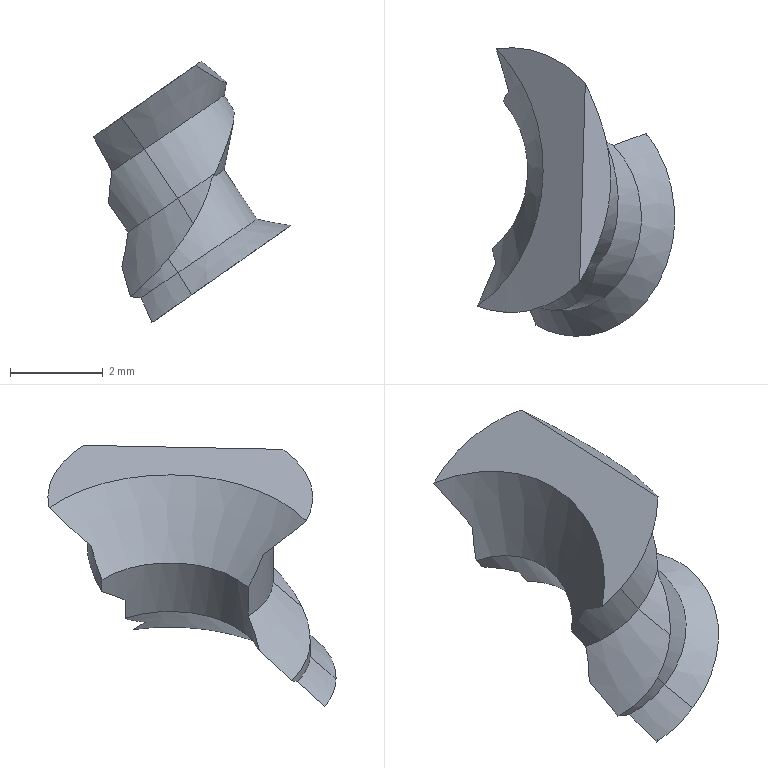Part | SolidWorks | features BaseBody 1 | 1 solid | 20 faces | box 4.246 x 6.208 x 5.627 mm | volume 24.691 mm3 | cone 11 | cylinder 6 | plane 3 | commonest cylinder face diameters 4 x6
STEP:
#1=CARTESIAN_POINT('',(-2079.786,537.162,-1636.577));
#2=VERTEX_POINT('',#1);
#3=CARTESIAN_POINT('',(-2078.265,541.527,-1635.512));
#4=VERTEX_POINT('',#3);
#5=CARTESIAN_POINT('',(-2079.786,537.162,-1636.577));
#6=CARTESIAN_POINT('',(-2079.49,537.155,-1636.37));
#7=CARTESIAN_POINT('',(-2079.24,537.225,-1636.195));
#8=CARTESIAN_POINT('',(-2078.948,537.352,-1635.991));
#9=CARTESIAN_POINT('',(-2078.864,537.398,-1635.931));
#10=CARTESIAN_POINT('',(-2078.755,537.466,-1635.855));
#11=CARTESIAN_POINT('',(-2078.722,537.489,-1635.832));
#12=CARTESIAN_POINT('',(-2078.677,537.521,-1635.8));
#13=CARTESIAN_POINT('',(-2078.655,537.537,-1635.785));
#14=CARTESIAN_POINT('',(-2078.631,537.555,-1635.768));
#15=CARTESIAN_POINT('',(-2078.62,537.564,-1635.76));
#16=CARTESIAN_POINT('',(-2078.615,537.568,-1635.757));
#17=CARTESIAN_POINT('',(-2078.612,537.57,-1635.755));
#18=CARTESIAN_POINT('',(-2078.612,537.57,-1635.755));
#19=CARTESIAN_POINT('',(-2078.419,537.723,-1635.62));
#20=CARTESIAN_POINT('',(-2078.258,537.904,-1635.507));
#21=CARTESIAN_POINT('',(-2078.061,538.198,-1635.369));
#22=CARTESIAN_POINT('',(-2078.003,538.299,-1635.328));
#23=CARTESIAN_POINT('',(-2077.926,538.455,-1635.275));
#24=CARTESIAN_POINT('',(-2077.903,538.507,-1635.258));
#25=CARTESIAN_POINT('',(-2077.87,538.586,-1635.235));
#26=CARTESIAN_POINT('',(-2077.854,538.626,-1635.224));
#27=CARTESIAN_POINT('',(-2077.839,538.665,-1635.214));
#28=CARTESIAN_POINT('',(-2077.829,538.692,-1635.207));
#29=CARTESIAN_POINT('',(-2077.825,538.704,-1635.204));
#30=CARTESIAN_POINT('',(-2077.738,538.953,-1635.143));
#31=CARTESIAN_POINT('',(-2077.686,539.201,-1635.106));
#32=CARTESIAN_POINT('',(-2077.653,539.579,-1635.084));
#33=CARTESIAN_POINT('',(-2077.65,539.706,-1635.082));
#34=CARTESIAN_POINT('',(-2077.657,539.895,-1635.086));
#35=CARTESIAN_POINT('',(-2077.663,539.989,-1635.091));
#36=CARTESIAN_POINT('',(-2077.676,540.098,-1635.099));
#37=CARTESIAN_POINT('',(-2077.682,540.145,-1635.104));
#38=CARTESIAN_POINT('',(-2077.686,540.176,-1635.107));
#39=CARTESIAN_POINT('',(-2077.689,540.193,-1635.109));
#40=CARTESIAN_POINT('',(-2077.727,540.434,-1635.135));
#41=CARTESIAN_POINT('',(-2077.79,540.666,-1635.18));
#42=CARTESIAN_POINT('',(-2077.98,541.116,-1635.313));
#43=CARTESIAN_POINT('',(-2078.106,541.333,-1635.401));
#44=CARTESIAN_POINT('',(-2078.265,541.527,-1635.512));
#45=B_SPLINE_CURVE_WITH_KNOTS('',3,(#5,#6,#7,#8,#9,#10,#11,#12,#13,#14,#15,#16,#17,#18,#19,#20,#21,#22,#23,#24,#25,#26,#27,#28,#29,#30,#31,#32,#33,#34,#35,#36,#37,#38,#39,#40,#41,#42,#43,#44),.UNSPECIFIED.,.F.,.F.,(4,2,2,2,1,1,1,2,2,2,2,2,1,2,2,2,2,1,1,2,2,2,4),(0.,0.125,0.1875,0.2188,0.2344,0.2422,0.2461,0.248,0.25,0.375,0.4375,0.4688,0.4844,0.4922,0.5,0.625,0.6875,0.7188,0.7344,0.7422,0.75,0.875,1.),.UNSPECIFIED.);
#46=EDGE_CURVE('',#2,#4,#45,.T.);
#47=ORIENTED_EDGE('',*,*,#46,.F.);
#48=CARTESIAN_POINT('',(-2080.638,537.403,-1637.174));
#49=VERTEX_POINT('',#48);
#50=CARTESIAN_POINT('',(-2080.638,537.403,-1637.174));
#51=CARTESIAN_POINT('',(-2080.371,537.25,-1636.987));
#52=CARTESIAN_POINT('',(-2080.079,537.168,-1636.782));
#53=CARTESIAN_POINT('',(-2079.786,537.162,-1636.577));
#54=B_SPLINE_CURVE_WITH_KNOTS('',3,(#50,#51,#52,#53),.UNSPECIFIED.,.F.,.F.,(4,4),(0.,1.),.UNSPECIFIED.);
#55=EDGE_CURVE('',#49,#2,#54,.T.);
#56=ORIENTED_EDGE('',*,*,#55,.F.);
#57=CARTESIAN_POINT('',(-2080.942,540.742,-1637.386));
#58=DIRECTION('',(0.5736,0.,-0.8192));
#59=DIRECTION('',(0.7965,0.2335,0.5577));
#60=AXIS2_PLACEMENT_3D('',#57,#58,#59);
#61=CIRCLE('',#60,3.36);
#62=EDGE_CURVE('',#4,#49,#61,.T.);
#63=ORIENTED_EDGE('',*,*,#62,.F.);
#64=EDGE_LOOP('',(#47,#56,#63));
#65=FACE_OUTER_BOUND('',#64,.T.);
#66=CARTESIAN_POINT('',(-2087.136,533.617,-1641.724));
#67=DIRECTION('',(0.5736,0.,-0.8192));
#68=DIRECTION('',(0.,-1.,0.));
#69=AXIS2_PLACEMENT_3D('',#66,#67,#68);
#70=PLANE('',#69);
#71=ADVANCED_FACE('',(#65),#70,.T.);
#72=CARTESIAN_POINT('',(-2078.976,541.269,-1635.356));
#73=VERTEX_POINT('',#72);
#74=CARTESIAN_POINT('',(-2080.286,541.707,-1635.267));
#75=VERTEX_POINT('',#74);
#76=CARTESIAN_POINT('',(-2078.976,541.269,-1635.356));
#77=CARTESIAN_POINT('',(-2079.333,541.497,-1635.327));
#78=CARTESIAN_POINT('',(-2079.782,541.661,-1635.306));
#79=CARTESIAN_POINT('',(-2080.286,541.707,-1635.267));
#80=B_SPLINE_CURVE_WITH_KNOTS('',3,(#76,#77,#78,#79),.UNSPECIFIED.,.F.,.F.,(4,4),(0.,1.),.UNSPECIFIED.);
#81=EDGE_CURVE('',#73,#75,#80,.T.);
#82=ORIENTED_EDGE('',*,*,#81,.F.);
#83=CARTESIAN_POINT('',(-2078.976,541.269,-1635.356));
#84=CARTESIAN_POINT('',(-2078.763,541.35,-1635.402));
#85=CARTESIAN_POINT('',(-2078.526,541.436,-1635.455));
#86=CARTESIAN_POINT('',(-2078.265,541.527,-1635.512));
#87=B_SPLINE_CURVE_WITH_KNOTS('',3,(#83,#84,#85,#86),.UNSPECIFIED.,.F.,.F.,(4,4),(0.,1.),.UNSPECIFIED.);
#88=EDGE_CURVE('',#73,#4,#87,.T.);
#89=ORIENTED_EDGE('',*,*,#88,.T.);
#90=ORIENTED_EDGE('',*,*,#62,.T.);
#91=CARTESIAN_POINT('',(-2080.873,538.001,-1636.635));
#92=VERTEX_POINT('',#91);
#93=CARTESIAN_POINT('',(-2080.873,538.001,-1636.635));
#94=CARTESIAN_POINT('',(-2080.806,537.825,-1636.792));
#95=CARTESIAN_POINT('',(-2080.728,537.626,-1636.971));
#96=CARTESIAN_POINT('',(-2080.638,537.403,-1637.174));
#97=B_SPLINE_CURVE_WITH_KNOTS('',3,(#93,#94,#95,#96),.UNSPECIFIED.,.F.,.F.,(4,4),(0.,1.),.UNSPECIFIED.);
#98=EDGE_CURVE('',#92,#49,#97,.T.);
#99=ORIENTED_EDGE('',*,*,#98,.F.);
#100=CARTESIAN_POINT('',(-2081.102,538.122,-1636.617));
#101=VERTEX_POINT('',#100);
#102=CARTESIAN_POINT('',(-2081.102,538.122,-1636.617));
#103=CARTESIAN_POINT('',(-2081.03,538.08,-1636.626));
#104=CARTESIAN_POINT('',(-2080.954,538.04,-1636.631));
#105=CARTESIAN_POINT('',(-2080.873,538.001,-1636.635));
#106=B_SPLINE_CURVE_WITH_KNOTS('',3,(#102,#103,#104,#105),.UNSPECIFIED.,.F.,.F.,(4,4),(0.,1.),.UNSPECIFIED.);
#107=EDGE_CURVE('',#101,#92,#106,.T.);
#108=ORIENTED_EDGE('',*,*,#107,.F.);
#109=CARTESIAN_POINT('',(-2081.286,538.814,-1635.967));
#110=VERTEX_POINT('',#109);
#111=CARTESIAN_POINT('',(-2081.286,538.814,-1635.967));
#112=CARTESIAN_POINT('',(-2081.234,538.608,-1636.153));
#113=CARTESIAN_POINT('',(-2081.172,538.377,-1636.369));
#114=CARTESIAN_POINT('',(-2081.102,538.122,-1636.617));
#115=B_SPLINE_CURVE_WITH_KNOTS('',3,(#111,#112,#113,#114),.UNSPECIFIED.,.F.,.F.,(4,4),(0.,1.),.UNSPECIFIED.);
#116=EDGE_CURVE('',#110,#101,#115,.T.);
#117=ORIENTED_EDGE('',*,*,#116,.F.);
#118=CARTESIAN_POINT('',(-2081.722,540.742,-1636.272));
#119=DIRECTION('',(0.5736,0.,-0.8192));
#120=DIRECTION('',(0.7176,0.4822,0.5025));
#121=AXIS2_PLACEMENT_3D('',#118,#119,#120);
#122=CIRCLE('',#121,2.);
#123=EDGE_CURVE('',#75,#110,#122,.T.);
#124=ORIENTED_EDGE('',*,*,#123,.F.);
#125=EDGE_LOOP('',(#82,#89,#90,#99,#108,#117,#124));
#126=FACE_OUTER_BOUND('',#125,.T.);
#127=CARTESIAN_POINT('',(-2081.761,540.742,-1636.216));
#128=DIRECTION('',(0.5736,0.,-0.8192));
#129=DIRECTION('',(-0.09983,-0.9925,-0.0699));
#130=AXIS2_PLACEMENT_3D('',#127,#128,#129);
#131=CONICAL_SURFACE('',#130,1.932,0.7854);
#132=ADVANCED_FACE('',(#126),#131,.F.);
#133=CARTESIAN_POINT('',(-2081.575,539.056,-1634.607));
#134=VERTEX_POINT('',#133);
#135=CARTESIAN_POINT('',(-2081.499,538.738,-1633.913));
#136=VERTEX_POINT('',#135);
#137=CARTESIAN_POINT('',(-2081.575,539.056,-1634.607));
#138=CARTESIAN_POINT('',(-2081.566,538.94,-1634.399));
#139=CARTESIAN_POINT('',(-2081.543,538.831,-1634.169));
#140=CARTESIAN_POINT('',(-2081.499,538.738,-1633.913));
#141=B_SPLINE_CURVE_WITH_KNOTS('',3,(#137,#138,#139,#140),.UNSPECIFIED.,.F.,.F.,(4,4),(0.,1.),.UNSPECIFIED.);
#142=EDGE_CURVE('',#134,#136,#141,.T.);
#143=ORIENTED_EDGE('',*,*,#142,.T.);
#144=CARTESIAN_POINT('',(-2081.899,537.805,-1633.174));
#145=VERTEX_POINT('',#144);
#146=CARTESIAN_POINT('',(-2081.899,537.805,-1633.174));
#147=CARTESIAN_POINT('',(-2081.74,538.164,-1633.468));
#148=CARTESIAN_POINT('',(-2081.607,538.475,-1633.715));
#149=CARTESIAN_POINT('',(-2081.499,538.738,-1633.913));
#150=B_SPLINE_CURVE_WITH_KNOTS('',3,(#146,#147,#148,#149),.UNSPECIFIED.,.F.,.F.,(4,4),(0.,1.),.UNSPECIFIED.);
#151=EDGE_CURVE('',#145,#136,#150,.T.);
#152=ORIENTED_EDGE('',*,*,#151,.F.);
#153=CARTESIAN_POINT('',(-2081.493,543.343,-1632.889));
#154=VERTEX_POINT('',#153);
#155=CARTESIAN_POINT('',(-2083.236,540.742,-1634.11));
#156=DIRECTION('',(-0.5736,0.,0.8192));
#157=DIRECTION('',(0.3978,-0.8742,0.2786));
#158=AXIS2_PLACEMENT_3D('',#155,#156,#157);
#159=CIRCLE('',#158,3.36);
#160=EDGE_CURVE('',#145,#154,#159,.T.);
#161=ORIENTED_EDGE('',*,*,#160,.T.);
#162=CARTESIAN_POINT('',(-2081.222,542.431,-1633.727));
#163=VERTEX_POINT('',#162);
#164=CARTESIAN_POINT('',(-2081.222,542.431,-1633.727));
#165=CARTESIAN_POINT('',(-2081.293,542.688,-1633.501));
#166=CARTESIAN_POINT('',(-2081.383,542.992,-1633.222));
#167=CARTESIAN_POINT('',(-2081.493,543.343,-1632.889));
#168=B_SPLINE_CURVE_WITH_KNOTS('',3,(#164,#165,#166,#167),.UNSPECIFIED.,.F.,.F.,(4,4),(0.,1.),.UNSPECIFIED.);
#169=EDGE_CURVE('',#163,#154,#168,.T.);
#170=ORIENTED_EDGE('',*,*,#169,.F.);
#171=CARTESIAN_POINT('',(-2081.337,542.203,-1634.44));
#172=VERTEX_POINT('',#171);
#173=CARTESIAN_POINT('',(-2081.222,542.431,-1633.727));
#174=CARTESIAN_POINT('',(-2081.276,542.373,-1633.987));
#175=CARTESIAN_POINT('',(-2081.313,542.293,-1634.224));
#176=CARTESIAN_POINT('',(-2081.337,542.203,-1634.44));
#177=B_SPLINE_CURVE_WITH_KNOTS('',3,(#173,#174,#175,#176),.UNSPECIFIED.,.F.,.F.,(4,4),(0.,1.),.UNSPECIFIED.);
#178=EDGE_CURVE('',#163,#172,#177,.T.);
#179=ORIENTED_EDGE('',*,*,#178,.T.);
#180=CARTESIAN_POINT('',(-2082.456,540.742,-1635.224));
#181=DIRECTION('',(-0.5736,0.,0.8192));
#182=DIRECTION('',(0.4404,-0.8432,0.3084));
#183=AXIS2_PLACEMENT_3D('',#180,#181,#182);
#184=CIRCLE('',#183,2.);
#185=EDGE_CURVE('',#134,#172,#184,.T.);
#186=ORIENTED_EDGE('',*,*,#185,.F.);
#187=EDGE_LOOP('',(#143,#152,#161,#170,#179,#186));
#188=FACE_OUTER_BOUND('',#187,.T.);
#189=CARTESIAN_POINT('',(-2082.417,540.742,-1635.279));
#190=DIRECTION('',(-0.5736,0.,0.8192));
#191=DIRECTION('',(-0.04287,0.9986,-0.03002));
#192=AXIS2_PLACEMENT_3D('',#189,#190,#191);
#193=CONICAL_SURFACE('',#192,1.932,0.7854);
#194=ADVANCED_FACE('',(#188),#193,.F.);
#195=CARTESIAN_POINT('',(-2081.163,542.205,-1634.693));
#196=VERTEX_POINT('',#195);
#197=CARTESIAN_POINT('',(-2081.337,542.203,-1634.44));
#198=CARTESIAN_POINT('',(-2081.279,542.204,-1634.525));
#199=CARTESIAN_POINT('',(-2081.221,542.205,-1634.609));
#200=CARTESIAN_POINT('',(-2081.163,542.205,-1634.693));
#201=B_SPLINE_CURVE_WITH_KNOTS('',3,(#197,#198,#199,#200),.UNSPECIFIED.,.F.,.F.,(4,4),(0.,1.),.UNSPECIFIED.);
#202=EDGE_CURVE('',#172,#196,#201,.T.);
#203=ORIENTED_EDGE('',*,*,#202,.T.);
#204=CARTESIAN_POINT('',(-2080.792,541.925,-1634.788));
#205=VERTEX_POINT('',#204);
#206=CARTESIAN_POINT('',(-2080.792,541.925,-1634.788));
#207=CARTESIAN_POINT('',(-2080.933,542.046,-1634.741));
#208=CARTESIAN_POINT('',(-2081.061,542.138,-1634.712));
#209=CARTESIAN_POINT('',(-2081.163,542.205,-1634.693));
#210=B_SPLINE_CURVE_WITH_KNOTS('',3,(#206,#207,#208,#209),.UNSPECIFIED.,.F.,.F.,(4,4),(0.,1.),.UNSPECIFIED.);
#211=EDGE_CURVE('',#205,#196,#210,.T.);
#212=ORIENTED_EDGE('',*,*,#211,.F.);
#213=CARTESIAN_POINT('',(-2080.559,541.708,-1634.879));
#214=VERTEX_POINT('',#213);
#215=CARTESIAN_POINT('',(-2080.559,541.708,-1634.879));
#216=CARTESIAN_POINT('',(-2080.632,541.781,-1634.846));
#217=CARTESIAN_POINT('',(-2080.71,541.854,-1634.815));
#218=CARTESIAN_POINT('',(-2080.792,541.925,-1634.788));
#219=B_SPLINE_CURVE_WITH_KNOTS('',3,(#215,#216,#217,#218),.UNSPECIFIED.,.F.,.F.,(4,4),(0.,1.),.UNSPECIFIED.);
#220=EDGE_CURVE('',#214,#205,#219,.T.);
#221=ORIENTED_EDGE('',*,*,#220,.F.);
#222=CARTESIAN_POINT('',(-2080.559,541.708,-1634.879));
#223=CARTESIAN_POINT('',(-2080.523,541.707,-1634.929));
#224=CARTESIAN_POINT('',(-2080.468,541.707,-1635.008));
#225=CARTESIAN_POINT('',(-2080.377,541.707,-1635.138));
#226=CARTESIAN_POINT('',(-2080.322,541.707,-1635.217));
#227=CARTESIAN_POINT('',(-2080.286,541.707,-1635.267));
#228=B_SPLINE_CURVE_WITH_KNOTS('',3,(#222,#223,#224,#225,#226,#227),.UNSPECIFIED.,.F.,.F.,(4,1,1,4),(0.,0.3889,0.6111,1.),.UNSPECIFIED.);
#229=EDGE_CURVE('',#214,#75,#228,.T.);
#230=ORIENTED_EDGE('',*,*,#229,.T.);
#231=ORIENTED_EDGE('',*,*,#123,.T.);
#232=CARTESIAN_POINT('',(-2081.153,539.051,-1635.224));
#233=VERTEX_POINT('',#232);
#234=CARTESIAN_POINT('',(-2081.286,538.814,-1635.967));
#235=CARTESIAN_POINT('',(-2081.263,538.835,-1635.868));
#236=CARTESIAN_POINT('',(-2081.23,538.874,-1635.714));
#237=CARTESIAN_POINT('',(-2081.186,538.954,-1635.465));
#238=CARTESIAN_POINT('',(-2081.164,539.011,-1635.317));
#239=CARTESIAN_POINT('',(-2081.153,539.051,-1635.224));
#240=B_SPLINE_CURVE_WITH_KNOTS('',3,(#234,#235,#236,#237,#238,#239),.UNSPECIFIED.,.F.,.F.,(4,1,1,4),(0.00001121,0.3929,0.615,1.),.UNSPECIFIED.);
#241=EDGE_CURVE('',#110,#233,#240,.T.);
#242=ORIENTED_EDGE('',*,*,#241,.T.);
#243=CARTESIAN_POINT('',(-2081.153,539.051,-1635.224));
#244=CARTESIAN_POINT('',(-2081.293,539.053,-1635.018));
#245=CARTESIAN_POINT('',(-2081.434,539.054,-1634.812));
#246=CARTESIAN_POINT('',(-2081.575,539.056,-1634.607));
#247=B_SPLINE_CURVE_WITH_KNOTS('',3,(#243,#244,#245,#246),.UNSPECIFIED.,.F.,.F.,(4,4),(0.,1.),.UNSPECIFIED.);
#248=EDGE_CURVE('',#233,#134,#247,.T.);
#249=ORIENTED_EDGE('',*,*,#248,.T.);
#250=ORIENTED_EDGE('',*,*,#185,.T.);
#251=EDGE_LOOP('',(#203,#212,#221,#230,#231,#242,#249,#250));
#252=FACE_OUTER_BOUND('',#251,.T.);
#253=CARTESIAN_POINT('',(-2081.685,540.742,-1636.325));
#254=DIRECTION('',(-0.5736,0.,0.8192));
#255=DIRECTION('',(-0.09983,-0.9925,-0.0699));
#256=AXIS2_PLACEMENT_3D('',#253,#254,#255);
#257=CYLINDRICAL_SURFACE('',#256,2.);
#258=ADVANCED_FACE('',(#252),#257,.F.);
#259=CARTESIAN_POINT('',(-2079.699,538.306,-1631.633));
#260=VERTEX_POINT('',#259);
#261=CARTESIAN_POINT('',(-2079.576,542.597,-1631.547));
#262=VERTEX_POINT('',#261);
#263=CARTESIAN_POINT('',(-2079.699,538.306,-1631.633));
#264=CARTESIAN_POINT('',(-2079.6,538.484,-1631.695));
#265=CARTESIAN_POINT('',(-2079.469,538.745,-1631.776));
#266=CARTESIAN_POINT('',(-2079.345,539.037,-1631.851));
#267=CARTESIAN_POINT('',(-2079.291,539.18,-1631.884));
#268=CARTESIAN_POINT('',(-2079.265,539.251,-1631.899));
#269=CARTESIAN_POINT('',(-2079.255,539.281,-1631.905));
#270=CARTESIAN_POINT('',(-2079.248,539.301,-1631.909));
#271=CARTESIAN_POINT('',(-2079.245,539.309,-1631.911));
#272=CARTESIAN_POINT('',(-2079.112,539.703,-1631.988));
#273=CARTESIAN_POINT('',(-2079.042,540.079,-1632.022));
#274=CARTESIAN_POINT('',(-2079.026,540.625,-1632.011));
#275=CARTESIAN_POINT('',(-2079.04,540.902,-1631.99));
#276=CARTESIAN_POINT('',(-2079.096,541.233,-1631.938));
#277=CARTESIAN_POINT('',(-2079.133,541.401,-1631.905));
#278=CARTESIAN_POINT('',(-2079.154,541.485,-1631.887));
#279=CARTESIAN_POINT('',(-2079.164,541.521,-1631.879));
#280=CARTESIAN_POINT('',(-2079.17,541.545,-1631.873));
#281=CARTESIAN_POINT('',(-2079.174,541.56,-1631.87));
#282=CARTESIAN_POINT('',(-2079.267,541.891,-1631.792));
#283=CARTESIAN_POINT('',(-2079.4,542.234,-1631.685));
#284=CARTESIAN_POINT('',(-2079.576,542.597,-1631.547));
#285=B_SPLINE_CURVE_WITH_KNOTS('',3,(#263,#264,#265,#266,#267,#268,#269,#270,#271,#272,#273,#274,#275,#276,#277,#278,#279,#280,#281,#282,#283,#284),.UNSPECIFIED.,.F.,.F.,(4,1,1,1,1,2,2,2,1,1,1,1,2,2,4),(0.,0.125,0.1875,0.2188,0.2344,0.2422,0.25,0.5,0.625,0.6875,0.7188,0.7344,0.7422,0.75,1.),.UNSPECIFIED.);
#286=EDGE_CURVE('',#260,#262,#285,.T.);
#287=ORIENTED_EDGE('',*,*,#286,.T.);
#288=CARTESIAN_POINT('',(-2079.699,538.306,-1631.633));
#289=DIRECTION('',(0.02859,0.9994,0.02002));
#290=VECTOR('',#289,1000.);
#291=LINE('',#288,#290);
#292=EDGE_CURVE('',#260,#262,#291,.T.);
#293=ORIENTED_EDGE('',*,*,#292,.F.);
#294=EDGE_LOOP('',(#287,#293));
#295=FACE_OUTER_BOUND('',#294,.T.);
#296=CARTESIAN_POINT('',(-2080.4,532.62,-1631.37));
#297=DIRECTION('',(0.5731,-0.03279,0.8188));
#298=DIRECTION('',(-0.05713,-0.9984,0.));
#299=AXIS2_PLACEMENT_3D('',#296,#297,#298);
#300=PLANE('',#299);
#301=ADVANCED_FACE('',(#295),#300,.T.);
#302=CARTESIAN_POINT('',(-2081.135,543.369,-1632.639));
#303=VERTEX_POINT('',#302);
#304=CARTESIAN_POINT('',(-2081.135,543.369,-1632.639));
#305=CARTESIAN_POINT('',(-2080.813,543.362,-1632.413));
#306=CARTESIAN_POINT('',(-2080.511,543.273,-1632.202));
#307=CARTESIAN_POINT('',(-2079.985,542.995,-1631.833));
#308=CARTESIAN_POINT('',(-2079.76,542.806,-1631.676));
#309=CARTESIAN_POINT('',(-2079.576,542.597,-1631.547));
#310=B_SPLINE_CURVE_WITH_KNOTS('',3,(#304,#305,#306,#307,#308,#309),.UNSPECIFIED.,.F.,.F.,(4,2,4),(0.,0.5,1.),.UNSPECIFIED.);
#311=EDGE_CURVE('',#303,#262,#310,.T.);
#312=ORIENTED_EDGE('',*,*,#311,.F.);
#313=CARTESIAN_POINT('',(-2081.493,543.343,-1632.889));
#314=CARTESIAN_POINT('',(-2081.447,543.35,-1632.857));
#315=CARTESIAN_POINT('',(-2081.374,543.36,-1632.806));
#316=CARTESIAN_POINT('',(-2081.255,543.369,-1632.722));
#317=CARTESIAN_POINT('',(-2081.182,543.37,-1632.671));
#318=CARTESIAN_POINT('',(-2081.135,543.369,-1632.639));
#319=B_SPLINE_CURVE_WITH_KNOTS('',3,(#313,#314,#315,#316,#317,#318),.UNSPECIFIED.,.F.,.F.,(4,1,1,4),(0.,0.3889,0.6111,1.),.UNSPECIFIED.);
#320=EDGE_CURVE('',#154,#303,#319,.T.);
#321=ORIENTED_EDGE('',*,*,#320,.F.);
#322=ORIENTED_EDGE('',*,*,#160,.F.);
#323=CARTESIAN_POINT('',(-2081.298,537.669,-1632.753));
#324=VERTEX_POINT('',#323);
#325=CARTESIAN_POINT('',(-2081.298,537.669,-1632.753));
#326=CARTESIAN_POINT('',(-2081.378,537.674,-1632.808));
#327=CARTESIAN_POINT('',(-2081.502,537.69,-1632.895));
#328=CARTESIAN_POINT('',(-2081.703,537.735,-1633.036));
#329=CARTESIAN_POINT('',(-2081.824,537.775,-1633.121));
#330=CARTESIAN_POINT('',(-2081.899,537.805,-1633.174));
#331=B_SPLINE_CURVE_WITH_KNOTS('',3,(#325,#326,#327,#328,#329,#330),.UNSPECIFIED.,.F.,.F.,(4,1,1,4),(0.00001607,0.3889,0.6111,1.),.UNSPECIFIED.);
#332=EDGE_CURVE('',#324,#145,#331,.T.);
#333=ORIENTED_EDGE('',*,*,#332,.F.);
#334=CARTESIAN_POINT('',(-2079.699,538.306,-1631.633));
#335=CARTESIAN_POINT('',(-2079.923,538.085,-1631.791));
#336=CARTESIAN_POINT('',(-2080.18,537.914,-1631.971));
#337=CARTESIAN_POINT('',(-2080.725,537.698,-1632.352));
#338=CARTESIAN_POINT('',(-2081.013,537.651,-1632.554));
#339=CARTESIAN_POINT('',(-2081.298,537.669,-1632.753));
#340=B_SPLINE_CURVE_WITH_KNOTS('',3,(#334,#335,#336,#337,#338,#339),.UNSPECIFIED.,.F.,.F.,(4,2,4),(0.,0.5,1.),.UNSPECIFIED.);
#341=EDGE_CURVE('',#260,#324,#340,.T.);
#342=ORIENTED_EDGE('',*,*,#341,.F.);
#343=ORIENTED_EDGE('',*,*,#292,.T.);
#344=EDGE_LOOP('',(#312,#321,#322,#333,#342,#343));
#345=FACE_OUTER_BOUND('',#344,.T.);
#346=CARTESIAN_POINT('',(-2079.331,533.263,-1631.375));
#347=DIRECTION('',(-0.5736,0.,0.8192));
#348=DIRECTION('',(0.,1.,0.));
#349=AXIS2_PLACEMENT_3D('',#346,#347,#348);
#350=PLANE('',#349);
#351=ADVANCED_FACE('',(#345),#350,.T.);
#352=CARTESIAN_POINT('',(-2080.683,542.516,-1633.363));
#353=VERTEX_POINT('',#352);
#354=CARTESIAN_POINT('',(-2080.477,542.516,-1633.668));
#355=VERTEX_POINT('',#354);
#356=CARTESIAN_POINT('',(-2080.683,542.516,-1633.363));
#357=DIRECTION('',(0.5592,0.,-0.829));
#358=VECTOR('',#357,1000.);
#359=LINE('',#356,#358);
#360=EDGE_CURVE('',#353,#355,#359,.T.);
#361=ORIENTED_EDGE('',*,*,#360,.T.);
#362=CARTESIAN_POINT('',(-2081.017,542.349,-1634.428));
#363=VERTEX_POINT('',#362);
#364=CARTESIAN_POINT('',(-2080.477,542.516,-1633.668));
#365=CARTESIAN_POINT('',(-2080.67,542.526,-1633.901));
#366=CARTESIAN_POINT('',(-2080.858,542.472,-1634.16));
#367=CARTESIAN_POINT('',(-2081.017,542.349,-1634.428));
#368=B_SPLINE_CURVE_WITH_KNOTS('',3,(#364,#365,#366,#367),.UNSPECIFIED.,.F.,.F.,(4,4),(0.,1.),.UNSPECIFIED.);
#369=EDGE_CURVE('',#355,#363,#368,.T.);
#370=ORIENTED_EDGE('',*,*,#369,.T.);
#371=CARTESIAN_POINT('',(-2081.017,542.349,-1634.428));
#372=CARTESIAN_POINT('',(-2081.068,542.309,-1634.513));
#373=CARTESIAN_POINT('',(-2081.117,542.262,-1634.602));
#374=CARTESIAN_POINT('',(-2081.163,542.205,-1634.693));
#375=B_SPLINE_CURVE_WITH_KNOTS('',3,(#371,#372,#373,#374),.UNSPECIFIED.,.F.,.F.,(4,4),(0.,1.),.UNSPECIFIED.);
#376=EDGE_CURVE('',#363,#196,#375,.T.);
#377=ORIENTED_EDGE('',*,*,#376,.T.);
#378=ORIENTED_EDGE('',*,*,#202,.F.);
#379=ORIENTED_EDGE('',*,*,#178,.F.);
#380=CARTESIAN_POINT('',(-2080.741,540.517,-1633.402));
#381=DIRECTION('',(-0.5592,0.,0.829));
#382=DIRECTION('',(0.02893,0.9994,0.01952));
#383=AXIS2_PLACEMENT_3D('',#380,#381,#382);
#384=CIRCLE('',#383,2.);
#385=EDGE_CURVE('',#353,#163,#384,.T.);
#386=ORIENTED_EDGE('',*,*,#385,.F.);
#387=EDGE_LOOP('',(#361,#370,#377,#378,#379,#386));
#388=FACE_OUTER_BOUND('',#387,.T.);
#389=CARTESIAN_POINT('',(-2079.989,540.517,-1634.516));
#390=DIRECTION('',(-0.5592,0.,0.829));
#391=DIRECTION('',(0.101,0.9925,0.06815));
#392=AXIS2_PLACEMENT_3D('',#389,#390,#391);
#393=CYLINDRICAL_SURFACE('',#392,2.);
#394=ADVANCED_FACE('',(#388),#393,.T.);
#395=ORIENTED_EDGE('',*,*,#169,.T.);
#396=ORIENTED_EDGE('',*,*,#320,.T.);
#397=CARTESIAN_POINT('',(-2081.135,543.369,-1632.639));
#398=DIRECTION('',(0.375,-0.7067,-0.6));
#399=VECTOR('',#398,1000.);
#400=LINE('',#397,#399);
#401=EDGE_CURVE('',#303,#353,#400,.T.);
#402=ORIENTED_EDGE('',*,*,#401,.T.);
#403=ORIENTED_EDGE('',*,*,#385,.T.);
#404=EDGE_LOOP('',(#395,#396,#402,#403));
#405=FACE_OUTER_BOUND('',#404,.T.);
#406=CARTESIAN_POINT('',(-2080.703,540.517,-1633.458));
#407=DIRECTION('',(-0.5592,0.,0.829));
#408=DIRECTION('',(0.04339,-0.9986,0.02927));
#409=AXIS2_PLACEMENT_3D('',#406,#407,#408);
#410=CONICAL_SURFACE('',#409,1.932,0.7854);
#411=ADVANCED_FACE('',(#405),#410,.T.);
#412=ORIENTED_EDGE('',*,*,#332,.T.);
#413=ORIENTED_EDGE('',*,*,#151,.T.);
#414=CARTESIAN_POINT('',(-2080.798,538.518,-1633.441));
#415=VERTEX_POINT('',#414);
#416=CARTESIAN_POINT('',(-2080.741,540.517,-1633.402));
#417=DIRECTION('',(-0.5592,0.,0.829));
#418=DIRECTION('',(-0.3791,-0.8893,-0.2557));
#419=AXIS2_PLACEMENT_3D('',#416,#417,#418);
#420=CIRCLE('',#419,2.);
#421=EDGE_CURVE('',#136,#415,#420,.T.);
#422=ORIENTED_EDGE('',*,*,#421,.T.);
#423=CARTESIAN_POINT('',(-2080.798,538.518,-1633.441));
#424=DIRECTION('',(-0.4159,-0.7067,0.5724));
#425=VECTOR('',#424,1000.);
#426=LINE('',#423,#425);
#427=EDGE_CURVE('',#415,#324,#426,.T.);
#428=ORIENTED_EDGE('',*,*,#427,.T.);
#429=EDGE_LOOP('',(#412,#413,#422,#428));
#430=FACE_OUTER_BOUND('',#429,.T.);
#431=CARTESIAN_POINT('',(-2080.703,540.517,-1633.458));
#432=DIRECTION('',(-0.5592,0.,0.829));
#433=DIRECTION('',(0.04339,-0.9986,0.02927));
#434=AXIS2_PLACEMENT_3D('',#431,#432,#433);
#435=CONICAL_SURFACE('',#434,1.932,0.7854);
#436=ADVANCED_FACE('',(#430),#435,.T.);
#437=ORIENTED_EDGE('',*,*,#401,.F.);
#438=ORIENTED_EDGE('',*,*,#311,.T.);
#439=ORIENTED_EDGE('',*,*,#286,.F.);
#440=ORIENTED_EDGE('',*,*,#341,.T.);
#441=ORIENTED_EDGE('',*,*,#427,.F.);
#442=CARTESIAN_POINT('',(-2080.741,540.517,-1633.402));
#443=DIRECTION('',(-0.5592,0.,0.829));
#444=DIRECTION('',(-0.02893,-0.9994,-0.01952));
#445=AXIS2_PLACEMENT_3D('',#442,#443,#444);
#446=CIRCLE('',#445,2.);
#447=EDGE_CURVE('',#415,#353,#446,.T.);
#448=ORIENTED_EDGE('',*,*,#447,.T.);
#449=EDGE_LOOP('',(#437,#438,#439,#440,#441,#448));
#450=FACE_OUTER_BOUND('',#449,.T.);
#451=CARTESIAN_POINT('',(-2080.703,540.517,-1633.458));
#452=DIRECTION('',(-0.5592,0.,0.829));
#453=DIRECTION('',(-0.04339,0.9986,-0.02927));
#454=AXIS2_PLACEMENT_3D('',#451,#452,#453);
#455=CONICAL_SURFACE('',#454,1.932,0.7854);
#456=ADVANCED_FACE('',(#450),#455,.T.);
#457=ORIENTED_EDGE('',*,*,#241,.F.);
#458=ORIENTED_EDGE('',*,*,#116,.T.);
#459=CARTESIAN_POINT('',(-2080.289,537.721,-1635.796));
#460=VERTEX_POINT('',#459);
#461=CARTESIAN_POINT('',(-2081.102,538.122,-1636.617));
#462=CARTESIAN_POINT('',(-2080.858,537.886,-1636.419));
#463=CARTESIAN_POINT('',(-2080.567,537.736,-1636.132));
#464=CARTESIAN_POINT('',(-2080.289,537.721,-1635.796));
#465=B_SPLINE_CURVE_WITH_KNOTS('',3,(#461,#462,#463,#464),.UNSPECIFIED.,.F.,.F.,(4,4),(0.,1.),.UNSPECIFIED.);
#466=EDGE_CURVE('',#101,#460,#465,.T.);
#467=ORIENTED_EDGE('',*,*,#466,.T.);
#468=CARTESIAN_POINT('',(-2079.748,537.888,-1635.037));
#469=VERTEX_POINT('',#468);
#470=CARTESIAN_POINT('',(-2080.289,537.721,-1635.796));
#471=CARTESIAN_POINT('',(-2080.102,537.711,-1635.571));
#472=CARTESIAN_POINT('',(-2079.91,537.762,-1635.31));
#473=CARTESIAN_POINT('',(-2079.748,537.888,-1635.037));
#474=B_SPLINE_CURVE_WITH_KNOTS('',3,(#470,#471,#472,#473),.UNSPECIFIED.,.F.,.F.,(4,4),(0.,1.),.UNSPECIFIED.);
#475=EDGE_CURVE('',#460,#469,#474,.T.);
#476=ORIENTED_EDGE('',*,*,#475,.T.);
#477=CARTESIAN_POINT('',(-2080.083,538.518,-1634.502));
#478=VERTEX_POINT('',#477);
#479=CARTESIAN_POINT('',(-2079.748,537.888,-1635.037));
#480=DIRECTION('',(-0.375,0.7067,0.6));
#481=VECTOR('',#480,1000.);
#482=LINE('',#479,#481);
#483=EDGE_CURVE('',#469,#478,#482,.T.);
#484=ORIENTED_EDGE('',*,*,#483,.T.);
#485=CARTESIAN_POINT('',(-2080.025,540.517,-1634.463));
#486=DIRECTION('',(0.5592,0.,-0.829));
#487=DIRECTION('',(-0.02893,-0.9994,-0.01952));
#488=AXIS2_PLACEMENT_3D('',#485,#486,#487);
#489=CIRCLE('',#488,2.);
#490=EDGE_CURVE('',#478,#233,#489,.T.);
#491=ORIENTED_EDGE('',*,*,#490,.T.);
#492=EDGE_LOOP('',(#457,#458,#467,#476,#484,#491));
#493=FACE_OUTER_BOUND('',#492,.T.);
#494=CARTESIAN_POINT('',(-2080.063,540.517,-1634.407));
#495=DIRECTION('',(0.5592,0.,-0.829));
#496=DIRECTION('',(0.101,0.9925,0.06815));
#497=AXIS2_PLACEMENT_3D('',#494,#495,#496);
#498=CONICAL_SURFACE('',#497,1.932,0.7854);
#499=ADVANCED_FACE('',(#493),#498,.T.);
#500=ORIENTED_EDGE('',*,*,#483,.F.);
#501=CARTESIAN_POINT('',(-2079.353,538.625,-1634.066));
#502=VERTEX_POINT('',#501);
#503=CARTESIAN_POINT('',(-2079.748,537.888,-1635.037));
#504=CARTESIAN_POINT('',(-2079.704,537.922,-1634.962));
#505=CARTESIAN_POINT('',(-2079.659,537.965,-1634.882));
#506=CARTESIAN_POINT('',(-2079.594,538.042,-1634.754));
#507=CARTESIAN_POINT('',(-2079.572,538.07,-1634.711));
#508=CARTESIAN_POINT('',(-2079.541,538.115,-1634.644));
#509=CARTESIAN_POINT('',(-2079.526,538.139,-1634.611));
#510=CARTESIAN_POINT('',(-2079.509,538.168,-1634.571));
#511=CARTESIAN_POINT('',(-2079.501,538.183,-1634.551));
#512=CARTESIAN_POINT('',(-2079.497,538.189,-1634.542));
#513=CARTESIAN_POINT('',(-2079.495,538.194,-1634.537));
#514=CARTESIAN_POINT('',(-2079.494,538.196,-1634.533));
#515=CARTESIAN_POINT('',(-2079.48,538.222,-1634.5));
#516=CARTESIAN_POINT('',(-2079.466,538.25,-1634.464));
#517=CARTESIAN_POINT('',(-2079.444,538.3,-1634.404));
#518=CARTESIAN_POINT('',(-2079.437,538.318,-1634.383));
#519=CARTESIAN_POINT('',(-2079.426,538.347,-1634.35));
#520=CARTESIAN_POINT('',(-2079.42,538.362,-1634.333));
#521=CARTESIAN_POINT('',(-2079.415,538.378,-1634.316));
#522=CARTESIAN_POINT('',(-2079.411,538.388,-1634.304));
#523=CARTESIAN_POINT('',(-2079.41,538.393,-1634.299));
#524=CARTESIAN_POINT('',(-2079.374,538.503,-1634.179));
#525=CARTESIAN_POINT('',(-2079.36,538.58,-1634.107));
#526=CARTESIAN_POINT('',(-2079.353,538.625,-1634.066));
#527=B_SPLINE_CURVE_WITH_KNOTS('',3,(#503,#504,#505,#506,#507,#508,#509,#510,#511,#512,#513,#514,#515,#516,#517,#518,#519,#520,#521,#522,#523,#524,#525,#526),.UNSPECIFIED.,.F.,.F.,(4,2,2,1,1,1,2,2,2,2,1,2,2,4),(0.,0.25,0.375,0.4375,0.4688,0.4844,0.4922,0.5,0.625,0.6875,0.7188,0.7344,0.75,1.),.UNSPECIFIED.);
#528=EDGE_CURVE('',#469,#502,#527,.T.);
#529=ORIENTED_EDGE('',*,*,#528,.T.);
#530=CARTESIAN_POINT('',(-2079.281,538.729,-1633.962));
#531=VERTEX_POINT('',#530);
#532=CARTESIAN_POINT('',(-2079.281,538.729,-1633.962));
#533=CARTESIAN_POINT('',(-2079.305,538.693,-1633.996));
#534=CARTESIAN_POINT('',(-2079.328,538.658,-1634.03));
#535=CARTESIAN_POINT('',(-2079.353,538.625,-1634.066));
#536=B_SPLINE_CURVE_WITH_KNOTS('',3,(#532,#533,#534,#535),.UNSPECIFIED.,.F.,.F.,(4,4),(0.,1.),.UNSPECIFIED.);
#537=EDGE_CURVE('',#531,#502,#536,.T.);
#538=ORIENTED_EDGE('',*,*,#537,.F.);
#539=CARTESIAN_POINT('',(-2080.025,540.517,-1634.463));
#540=DIRECTION('',(0.5592,0.,-0.829));
#541=DIRECTION('',(0.3718,-0.8938,0.2508));
#542=AXIS2_PLACEMENT_3D('',#539,#540,#541);
#543=CIRCLE('',#542,2.);
#544=EDGE_CURVE('',#531,#478,#543,.T.);
#545=ORIENTED_EDGE('',*,*,#544,.T.);
#546=EDGE_LOOP('',(#500,#529,#538,#545));
#547=FACE_OUTER_BOUND('',#546,.T.);
#548=CARTESIAN_POINT('',(-2080.063,540.517,-1634.407));
#549=DIRECTION('',(0.5592,0.,-0.829));
#550=DIRECTION('',(-0.101,-0.9925,-0.06815));
#551=AXIS2_PLACEMENT_3D('',#548,#549,#550);
#552=CONICAL_SURFACE('',#551,1.932,0.7854);
#553=ADVANCED_FACE('',(#547),#552,.T.);
#554=CARTESIAN_POINT('',(-2080.083,538.518,-1634.502));
#555=DIRECTION('',(-0.5592,0.,0.829));
#556=VECTOR('',#555,1000.);
#557=LINE('',#554,#556);
#558=EDGE_CURVE('',#478,#415,#557,.T.);
#559=ORIENTED_EDGE('',*,*,#558,.F.);
#560=ORIENTED_EDGE('',*,*,#544,.F.);
#561=CARTESIAN_POINT('',(-2079.281,538.729,-1633.962));
#562=CARTESIAN_POINT('',(-2079.187,538.829,-1633.746));
#563=CARTESIAN_POINT('',(-2079.107,538.957,-1633.554));
#564=CARTESIAN_POINT('',(-2079.013,539.175,-1633.305));
#565=CARTESIAN_POINT('',(-2078.986,539.251,-1633.228));
#566=CARTESIAN_POINT('',(-2078.952,539.37,-1633.123));
#567=CARTESIAN_POINT('',(-2078.936,539.43,-1633.072));
#568=CARTESIAN_POINT('',(-2078.921,539.502,-1633.018));
#569=CARTESIAN_POINT('',(-2078.914,539.538,-1632.991));
#570=CARTESIAN_POINT('',(-2078.911,539.554,-1632.98));
#571=CARTESIAN_POINT('',(-2078.909,539.564,-1632.973));
#572=CARTESIAN_POINT('',(-2078.908,539.568,-1632.97));
#573=CARTESIAN_POINT('',(-2078.872,539.774,-1632.827));
#574=CARTESIAN_POINT('',(-2078.86,539.988,-1632.719));
#575=CARTESIAN_POINT('',(-2078.876,540.312,-1632.604));
#576=CARTESIAN_POINT('',(-2078.887,540.42,-1632.573));
#577=CARTESIAN_POINT('',(-2078.911,540.582,-1632.538));
#578=CARTESIAN_POINT('',(-2078.925,540.662,-1632.524));
#579=CARTESIAN_POINT('',(-2078.945,540.754,-1632.511));
#580=CARTESIAN_POINT('',(-2078.955,540.794,-1632.507));
#581=CARTESIAN_POINT('',(-2078.961,540.82,-1632.505));
#582=CARTESIAN_POINT('',(-2078.964,540.832,-1632.503));
#583=CARTESIAN_POINT('',(-2079.026,541.075,-1632.484));
#584=CARTESIAN_POINT('',(-2079.11,541.296,-1632.5));
#585=CARTESIAN_POINT('',(-2079.266,541.597,-1632.571));
#586=CARTESIAN_POINT('',(-2079.323,541.693,-1632.603));
#587=CARTESIAN_POINT('',(-2079.414,541.826,-1632.662));
#588=CARTESIAN_POINT('',(-2079.446,541.869,-1632.683));
#589=CARTESIAN_POINT('',(-2079.511,541.951,-1632.729));
#590=CARTESIAN_POINT('',(-2079.545,541.991,-1632.754));
#591=CARTESIAN_POINT('',(-2079.713,542.174,-1632.883));
#592=CARTESIAN_POINT('',(-2079.86,542.293,-1633.013));
#593=CARTESIAN_POINT('',(-2080.166,542.46,-1633.313));
#594=CARTESIAN_POINT('',(-2080.324,542.508,-1633.484));
#595=CARTESIAN_POINT('',(-2080.477,542.516,-1633.668));
#596=B_SPLINE_CURVE_WITH_KNOTS('',3,(#561,#562,#563,#564,#565,#566,#567,#568,#569,#570,#571,#572,#573,#574,#575,#576,#577,#578,#579,#580,#581,#582,#583,#584,#585,#586,#587,#588,#589,#590,#591,#592,#593,#594,#595),.UNSPECIFIED.,.F.,.F.,(4,2,2,1,1,1,2,2,2,2,1,1,2,2,2,2,2,2,2,4),(0.,0.125,0.1875,0.2187,0.2344,0.2422,0.2461,0.25,0.375,0.4375,0.4687,0.4844,0.4922,0.5,0.625,0.6875,0.7187,0.75,0.875,1.),.UNSPECIFIED.);
#597=EDGE_CURVE('',#531,#355,#596,.T.);
#598=ORIENTED_EDGE('',*,*,#597,.T.);
#599=ORIENTED_EDGE('',*,*,#360,.F.);
#600=ORIENTED_EDGE('',*,*,#447,.F.);
#601=EDGE_LOOP('',(#559,#560,#598,#599,#600));
#602=FACE_OUTER_BOUND('',#601,.T.);
#603=CARTESIAN_POINT('',(-2079.989,540.517,-1634.516));
#604=DIRECTION('',(-0.5592,0.,0.829));
#605=DIRECTION('',(-0.101,-0.9925,-0.06815));
#606=AXIS2_PLACEMENT_3D('',#603,#604,#605);
#607=CYLINDRICAL_SURFACE('',#606,2.);
#608=ADVANCED_FACE('',(#602),#607,.T.);
#609=ORIENTED_EDGE('',*,*,#558,.T.);
#610=ORIENTED_EDGE('',*,*,#421,.F.);
#611=ORIENTED_EDGE('',*,*,#142,.F.);
#612=ORIENTED_EDGE('',*,*,#248,.F.);
#613=ORIENTED_EDGE('',*,*,#490,.F.);
#614=EDGE_LOOP('',(#609,#610,#611,#612,#613));
#615=FACE_OUTER_BOUND('',#614,.T.);
#616=CARTESIAN_POINT('',(-2079.989,540.517,-1634.516));
#617=DIRECTION('',(-0.5592,0.,0.829));
#618=DIRECTION('',(0.101,0.9925,0.06815));
#619=AXIS2_PLACEMENT_3D('',#616,#617,#618);
#620=CYLINDRICAL_SURFACE('',#619,2.);
#621=ADVANCED_FACE('',(#615),#620,.T.);
#622=CARTESIAN_POINT('',(-2080.083,537.721,-1636.102));
#623=VERTEX_POINT('',#622);
#624=CARTESIAN_POINT('',(-2079.786,537.162,-1636.577));
#625=DIRECTION('',(-0.375,0.7067,0.6));
#626=VECTOR('',#625,1000.);
#627=LINE('',#624,#626);
#628=EDGE_CURVE('',#2,#623,#627,.T.);
#629=ORIENTED_EDGE('',*,*,#628,.F.);
#630=ORIENTED_EDGE('',*,*,#46,.T.);
#631=ORIENTED_EDGE('',*,*,#88,.F.);
#632=CARTESIAN_POINT('',(-2080.025,539.72,-1636.063));
#633=DIRECTION('',(0.5592,0.,-0.829));
#634=DIRECTION('',(0.5242,0.7747,0.3536));
#635=AXIS2_PLACEMENT_3D('',#632,#633,#634);
#636=CIRCLE('',#635,2.);
#637=EDGE_CURVE('',#73,#623,#636,.T.);
#638=ORIENTED_EDGE('',*,*,#637,.T.);
#639=EDGE_LOOP('',(#629,#630,#631,#638));
#640=FACE_OUTER_BOUND('',#639,.T.);
#641=CARTESIAN_POINT('',(-2080.063,539.72,-1636.007));
#642=DIRECTION('',(0.5592,0.,-0.829));
#643=DIRECTION('',(-0.101,-0.9925,-0.06815));
#644=AXIS2_PLACEMENT_3D('',#641,#642,#643);
#645=CONICAL_SURFACE('',#644,1.932,0.7854);
#646=ADVANCED_FACE('',(#640),#645,.T.);
#647=ORIENTED_EDGE('',*,*,#220,.T.);
#648=CARTESIAN_POINT('',(-2081.017,542.349,-1634.428));
#649=DIRECTION('',(0.375,-0.7067,-0.6));
#650=VECTOR('',#649,1000.);
#651=LINE('',#648,#650);
#652=EDGE_CURVE('',#363,#205,#651,.T.);
#653=ORIENTED_EDGE('',*,*,#652,.F.);
#654=ORIENTED_EDGE('',*,*,#369,.F.);
#655=ORIENTED_EDGE('',*,*,#597,.F.);
#656=ORIENTED_EDGE('',*,*,#537,.T.);
#657=CARTESIAN_POINT('',(-2080.741,539.72,-1635.002));
#658=DIRECTION('',(-0.5592,0.,0.829));
#659=DIRECTION('',(0.6939,-0.5472,0.4681));
#660=AXIS2_PLACEMENT_3D('',#657,#658,#659);
#661=CIRCLE('',#660,2.);
#662=EDGE_CURVE('',#502,#214,#661,.T.);
#663=ORIENTED_EDGE('',*,*,#662,.T.);
#664=EDGE_LOOP('',(#647,#653,#654,#655,#656,#663));
#665=FACE_OUTER_BOUND('',#664,.T.);
#666=CARTESIAN_POINT('',(-2080.703,539.72,-1635.058));
#667=DIRECTION('',(-0.5592,0.,0.829));
#668=DIRECTION('',(-0.04339,0.9986,-0.02927));
#669=AXIS2_PLACEMENT_3D('',#666,#667,#668);
#670=CONICAL_SURFACE('',#669,1.932,0.7854);
#671=ADVANCED_FACE('',(#665),#670,.T.);
#672=ORIENTED_EDGE('',*,*,#528,.F.);
#673=ORIENTED_EDGE('',*,*,#475,.F.);
#674=CARTESIAN_POINT('',(-2080.083,537.721,-1636.102));
#675=DIRECTION('',(-0.5592,0.,0.829));
#676=VECTOR('',#675,1000.);
#677=LINE('',#674,#676);
#678=EDGE_CURVE('',#623,#460,#677,.T.);
#679=ORIENTED_EDGE('',*,*,#678,.F.);
#680=ORIENTED_EDGE('',*,*,#637,.F.);
#681=ORIENTED_EDGE('',*,*,#81,.T.);
#682=ORIENTED_EDGE('',*,*,#229,.F.);
#683=ORIENTED_EDGE('',*,*,#662,.F.);
#684=EDGE_LOOP('',(#672,#673,#679,#680,#681,#682,#683));
#685=FACE_OUTER_BOUND('',#684,.T.);
#686=CARTESIAN_POINT('',(-2079.989,539.72,-1636.116));
#687=DIRECTION('',(-0.5592,0.,0.829));
#688=DIRECTION('',(-0.101,-0.9925,-0.06815));
#689=AXIS2_PLACEMENT_3D('',#686,#687,#688);
#690=CYLINDRICAL_SURFACE('',#689,2.);
#691=ADVANCED_FACE('',(#685),#690,.T.);
#692=ORIENTED_EDGE('',*,*,#98,.T.);
#693=ORIENTED_EDGE('',*,*,#55,.T.);
#694=ORIENTED_EDGE('',*,*,#628,.T.);
#695=CARTESIAN_POINT('',(-2080.025,539.72,-1636.063));
#696=DIRECTION('',(0.5592,0.,-0.829));
#697=DIRECTION('',(-0.02893,-0.9994,-0.01952));
#698=AXIS2_PLACEMENT_3D('',#695,#696,#697);
#699=CIRCLE('',#698,2.);
#700=EDGE_CURVE('',#623,#92,#699,.T.);
#701=ORIENTED_EDGE('',*,*,#700,.T.);
#702=EDGE_LOOP('',(#692,#693,#694,#701));
#703=FACE_OUTER_BOUND('',#702,.T.);
#704=CARTESIAN_POINT('',(-2080.063,539.72,-1636.007));
#705=DIRECTION('',(0.5592,0.,-0.829));
#706=DIRECTION('',(0.101,0.9925,0.06815));
#707=AXIS2_PLACEMENT_3D('',#704,#705,#706);
#708=CONICAL_SURFACE('',#707,1.932,0.7854);
#709=ADVANCED_FACE('',(#703),#708,.T.);
#710=ORIENTED_EDGE('',*,*,#211,.T.);
#711=ORIENTED_EDGE('',*,*,#376,.F.);
#712=ORIENTED_EDGE('',*,*,#652,.T.);
#713=EDGE_LOOP('',(#710,#711,#712));
#714=FACE_OUTER_BOUND('',#713,.T.);
#715=CARTESIAN_POINT('',(-2080.703,539.72,-1635.058));
#716=DIRECTION('',(-0.5592,0.,0.829));
#717=DIRECTION('',(0.04339,-0.9986,0.02927));
#718=AXIS2_PLACEMENT_3D('',#715,#716,#717);
#719=CONICAL_SURFACE('',#718,1.932,0.7854);
#720=ADVANCED_FACE('',(#714),#719,.T.);
#721=ORIENTED_EDGE('',*,*,#678,.T.);
#722=ORIENTED_EDGE('',*,*,#466,.F.);
#723=ORIENTED_EDGE('',*,*,#107,.T.);
#724=ORIENTED_EDGE('',*,*,#700,.F.);
#725=EDGE_LOOP('',(#721,#722,#723,#724));
#726=FACE_OUTER_BOUND('',#725,.T.);
#727=CARTESIAN_POINT('',(-2079.989,539.72,-1636.116));
#728=DIRECTION('',(-0.5592,0.,0.829));
#729=DIRECTION('',(0.101,0.9925,0.06815));
#730=AXIS2_PLACEMENT_3D('',#727,#728,#729);
#731=CYLINDRICAL_SURFACE('',#730,2.);
#732=ADVANCED_FACE('',(#726),#731,.T.);
#733=CLOSED_SHELL('',(#71,#132,#194,#258,#301,#351,#394,#411,#436,#456,#499,#553,#608,#621,#646,#671,#691,#709,#720,#732));
#734=MANIFOLD_SOLID_BREP('',#733);
#735=CARTESIAN_POINT('',(0.,0.,0.));
#736=DIRECTION('',(0.,0.,1.));
#737=DIRECTION('',(1.,0.,0.));
#738=AXIS2_PLACEMENT_3D('',#735,#736,#737);
#739=(LENGTH_UNIT()NAMED_UNIT(*)SI_UNIT(.MILLI.,.METRE.));
#740=UNCERTAINTY_MEASURE_WITH_UNIT(LENGTH_MEASURE(0.00001),#739,'','');
#741=(NAMED_UNIT(*)PLANE_ANGLE_UNIT()SI_UNIT($,.RADIAN.));
#742=(NAMED_UNIT(*)SI_UNIT($,.STERADIAN.)SOLID_ANGLE_UNIT());
#743=(GEOMETRIC_REPRESENTATION_CONTEXT(3)GLOBAL_UNCERTAINTY_ASSIGNED_CONTEXT((#740))GLOBAL_UNIT_ASSIGNED_CONTEXT((#739,#741,#742))REPRESENTATION_CONTEXT('',''));
#744=ADVANCED_BREP_SHAPE_REPRESENTATION('',(#734,#738),#743);